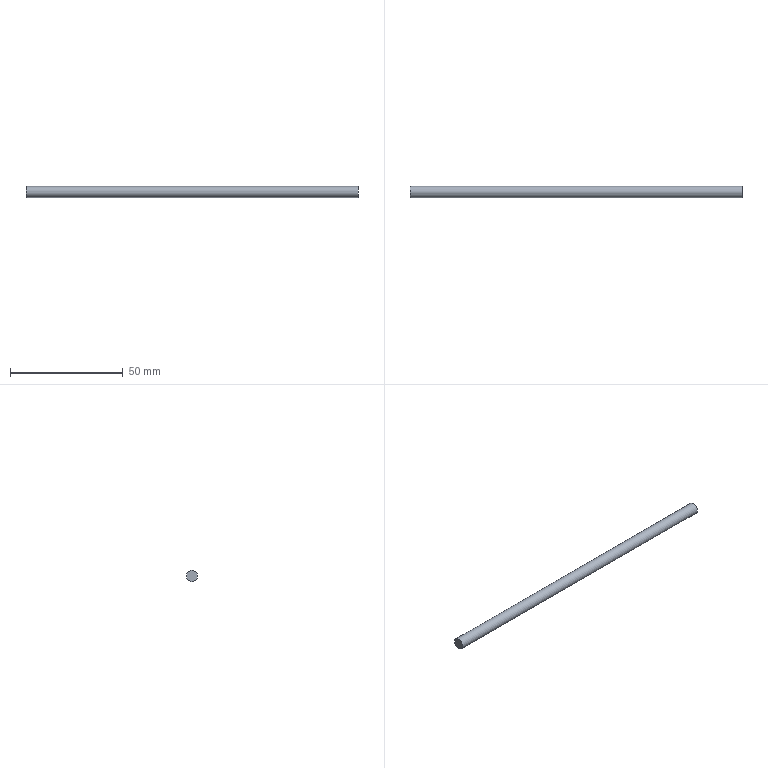Part | NX | features solid 2 | 1 solid | 3 faces | box 147 x 5 x 5 mm | volume 2886 mm3 | plane 2 | cylinder 1 | commonest cylinder face diameters 5 x1
STEP:
#1=CARTESIAN_POINT('',(65.,-377.5,-412.5));
#2=VERTEX_POINT('',#1);
#3=CARTESIAN_POINT('',(65.,-377.5,-410.));
#4=DIRECTION('',(1.,0.,0.));
#5=DIRECTION('',(0.,0.,-1.));
#6=AXIS2_PLACEMENT_3D('',#3,#4,#5);
#7=CIRCLE('',#6,2.5);
#8=EDGE_CURVE('',#2,#2,#7,.T.);
#9=ORIENTED_EDGE('',*,*,#8,.T.);
#10=EDGE_LOOP('',(#9));
#11=FACE_BOUND('',#10,.T.);
#12=CARTESIAN_POINT('',(212.,-377.5,-407.5));
#13=VERTEX_POINT('',#12);
#14=CARTESIAN_POINT('',(212.,-377.5,-410.));
#15=DIRECTION('',(1.,0.,0.));
#16=DIRECTION('',(0.,0.,1.));
#17=AXIS2_PLACEMENT_3D('',#14,#15,#16);
#18=CIRCLE('',#17,2.5);
#19=EDGE_CURVE('',#13,#13,#18,.T.);
#20=ORIENTED_EDGE('',*,*,#19,.F.);
#21=EDGE_LOOP('',(#20));
#22=FACE_BOUND('',#21,.T.);
#23=CARTESIAN_POINT('',(52.,-377.5,-410.));
#24=DIRECTION('',(1.,0.,0.));
#25=DIRECTION('',(0.,0.,-1.));
#26=AXIS2_PLACEMENT_3D('',#23,#24,#25);
#27=CYLINDRICAL_SURFACE('',#26,2.5);
#28=ADVANCED_FACE('',(#11,#22),#27,.T.);
#29=ORIENTED_EDGE('',*,*,#8,.F.);
#30=EDGE_LOOP('',(#29));
#31=FACE_BOUND('',#30,.T.);
#32=CARTESIAN_POINT('',(65.,80.624,-300.));
#33=DIRECTION('',(1.,0.,0.));
#34=DIRECTION('',(0.,0.,-1.));
#35=AXIS2_PLACEMENT_3D('',#32,#33,#34);
#36=PLANE('',#35);
#37=ADVANCED_FACE('',(#31),#36,.F.);
#38=ORIENTED_EDGE('',*,*,#19,.T.);
#39=EDGE_LOOP('',(#38));
#40=FACE_BOUND('',#39,.T.);
#41=CARTESIAN_POINT('',(212.,-377.5,-410.));
#42=DIRECTION('',(-1.,0.,0.));
#43=DIRECTION('',(0.,0.,1.));
#44=AXIS2_PLACEMENT_3D('',#41,#42,#43);
#45=PLANE('',#44);
#46=ADVANCED_FACE('',(#40),#45,.F.);
#47=CLOSED_SHELL('',(#28,#37,#46));
#48=MANIFOLD_SOLID_BREP('',#47);
#49=(LENGTH_UNIT()NAMED_UNIT(*)SI_UNIT(.MILLI.,.METRE.));
#50=UNCERTAINTY_MEASURE_WITH_UNIT(LENGTH_MEASURE(0.00001),#49,'','');
#51=(NAMED_UNIT(*)PLANE_ANGLE_UNIT()SI_UNIT($,.RADIAN.));
#52=(NAMED_UNIT(*)SI_UNIT($,.STERADIAN.)SOLID_ANGLE_UNIT());
#53=(GEOMETRIC_REPRESENTATION_CONTEXT(3)GLOBAL_UNCERTAINTY_ASSIGNED_CONTEXT((#50))GLOBAL_UNIT_ASSIGNED_CONTEXT((#49,#51,#52))REPRESENTATION_CONTEXT('',''));
#54=ADVANCED_BREP_SHAPE_REPRESENTATION('',(#48),#53);